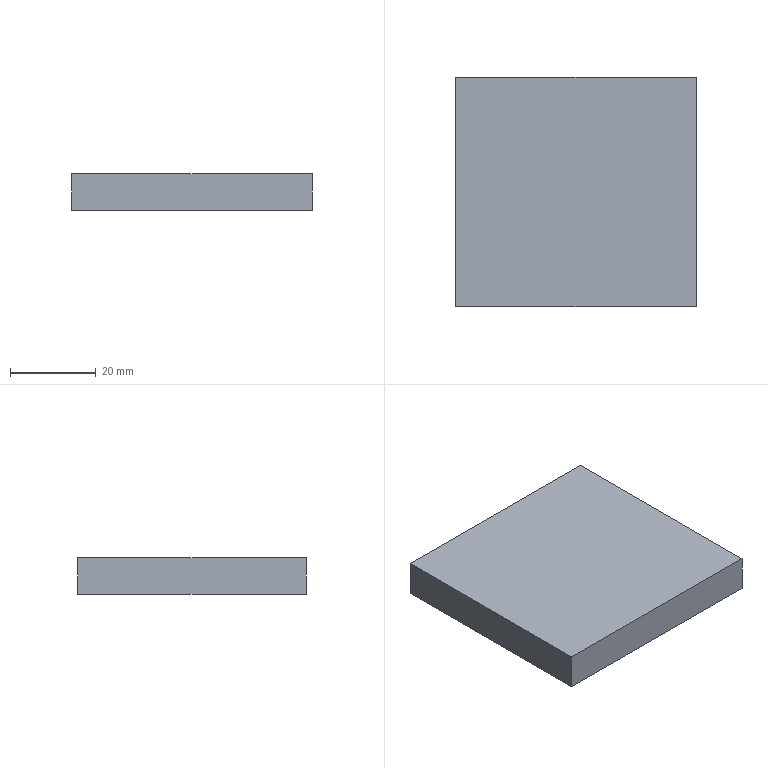NC program | NX | posted with a generic post | part box 56 x 53.3 x 8.5 mm
Lines 2013 to 2943 of 2943:
(ZLEVEL_PROFILE_COPY_COPY_COPY , TOOL : D2)
N4018 T18 M6
N4020 G54
N4022 G17 G0 G90 X19.843 Y-6.394 S9500 M3
N4024 G43 Z30. H18
N4026 Z-0.146
N4028 G94 G1 X20.091 Y-6.597 F1000.
N4030 G3 X20.288 Y-6.629 R0.2
N4032 G2 X21.018 Y-6.5 R2. F1100.
N4034 G3 X21.241 Y-5.728 R22.
N4036 X21.19 Y-5.534 R0.2
N4038 G1 X20.943 Y-5.287
N4040 G0 X19.843 Y-6.394 Z-0.292
N4042 G1 X20.091 Y-6.597 F1000.
N4044 G3 X20.288 Y-6.629 R0.2
N4046 G2 X21.018 Y-6.5 R2. F1100.
N4048 G3 X21.241 Y-5.728 R22.
N4050 X21.19 Y-5.534 R0.2
N4052 G1 X20.943 Y-5.287
N4054 G0 X19.843 Y-6.394 Z-0.438
N4056 G1 X20.091 Y-6.597 F1000.
N4058 G3 X20.288 Y-6.629 R0.2
N4060 G2 X21.018 Y-6.5 R2. F1100.
N4062 G3 X21.241 Y-5.728 R22.
N4064 X21.19 Y-5.534 R0.2
N4066 G1 X20.943 Y-5.287
N4068 G0 X19.843 Y-6.394 Z-0.583
N4070 G1 X20.091 Y-6.597 F1000.
N4072 G3 X20.288 Y-6.629 R0.2
N4074 G2 X21.018 Y-6.5 R2. F1100.
N4076 G3 X21.241 Y-5.728 R22.
N4078 X21.19 Y-5.534 R0.2
N4080 G1 X20.943 Y-5.287
N4082 G0 X19.843 Y-6.394 Z-0.729
N4084 G1 X20.091 Y-6.597 F1000.
N4086 G3 X20.288 Y-6.629 R0.2
N4088 G2 X21.018 Y-6.5 R2. F1100.
N4090 G3 X21.241 Y-5.728 R22.
N4092 X21.19 Y-5.534 R0.2
N4094 G1 X20.943 Y-5.287
N4096 G0 X19.843 Y-6.394 Z-0.875
N4098 G1 X20.091 Y-6.597 F1000.
N4100 G3 X20.288 Y-6.629 R0.2
N4102 G2 X21.018 Y-6.5 R2. F1100.
N4104 G3 X21.241 Y-5.728 R22.
N4106 X21.19 Y-5.534 R0.2
N4108 G1 X20.943 Y-5.287
N4110 G0 X19.843 Y-6.394 Z-1.021
N4112 G1 X20.091 Y-6.597 F1000.
N4114 G3 X20.288 Y-6.629 R0.2
N4116 G2 X21.018 Y-6.5 R2. F1100.
N4118 G3 X21.241 Y-5.728 R22.
N4120 X21.19 Y-5.534 R0.2
N4122 G1 X20.943 Y-5.287
N4124 G0 X19.843 Y-6.394 Z-1.167
N4126 G1 X20.091 Y-6.597 F1000.
N4128 G3 X20.288 Y-6.629 R0.2
N4130 G2 X21.018 Y-6.5 R2. F1100.
N4132 G3 X21.241 Y-5.728 R22.
N4134 X21.19 Y-5.534 R0.2
N4136 G1 X20.943 Y-5.287
N4138 G0 X19.843 Y-6.394 Z-1.313
N4140 G1 X20.091 Y-6.597 F1000.
N4142 G3 X20.288 Y-6.629 R0.2
N4144 G2 X21.018 Y-6.5 R2. F1100.
N4146 G3 X21.241 Y-5.728 R22.
N4148 X21.19 Y-5.534 R0.2
N4150 G1 X20.943 Y-5.287
N4152 G0 X19.843 Y-6.394 Z-1.458
N4154 G1 X20.091 Y-6.597 F1000.
N4156 G3 X20.288 Y-6.629 R0.2
N4158 G2 X21.018 Y-6.5 R2. F1100.
N4160 G3 X21.241 Y-5.728 R22.
N4162 X21.19 Y-5.534 R0.2
N4164 G1 X20.943 Y-5.287
N4166 G0 X19.843 Y-6.394 Z-1.604
N4168 G1 X20.091 Y-6.597 F1000.
N4170 G3 X20.288 Y-6.629 R0.2
N4172 G2 X21.018 Y-6.5 R2. F1100.
N4174 G3 X21.241 Y-5.728 R22.
N4176 X21.19 Y-5.534 R0.2
N4178 G1 X20.943 Y-5.287
N4180 G0 X19.843 Y-6.394 Z-1.75
N4182 G1 X20.091 Y-6.597 F1000.
N4184 G3 X20.288 Y-6.629 R0.2
N4186 G2 X21.018 Y-6.5 R2. F1100.
N4188 G3 X21.241 Y-5.728 R22.
N4190 X21.19 Y-5.534 R0.2
N4192 G1 X20.943 Y-5.287
N4194 G0 X19.843 Y-6.394 Z-1.896
N4196 G1 X20.091 Y-6.597 F1000.
N4198 G3 X20.288 Y-6.629 R0.2
N4200 G2 X21.018 Y-6.5 R2. F1100.
N4202 G3 X21.241 Y-5.728 R22.
N4204 X21.19 Y-5.534 R0.2
N4206 G1 X20.943 Y-5.287
N4208 G0 X19.843 Y-6.394 Z-2.042
N4210 G1 X20.091 Y-6.597 F1000.
N4212 G3 X20.288 Y-6.629 R0.2
N4214 G2 X21.018 Y-6.5 R2. F1100.
N4216 G3 X21.241 Y-5.728 R22.
N4218 X21.19 Y-5.534 R0.2
N4220 G1 X20.943 Y-5.287
N4222 G0 X19.843 Y-6.394 Z-2.188
N4224 G1 X20.091 Y-6.597 F1000.
N4226 G3 X20.288 Y-6.629 R0.2
N4228 G2 X21.018 Y-6.5 R2. F1100.
N4230 G3 X21.241 Y-5.728 R22.
N4232 X21.19 Y-5.534 R0.2
N4234 G1 X20.943 Y-5.287
N4236 G0 X19.843 Y-6.394 Z-2.333
N4238 G1 X20.091 Y-6.597 F1000.
N4240 G3 X20.288 Y-6.629 R0.2
N4242 G2 X21.018 Y-6.5 R2. F1100.
N4244 G3 X21.241 Y-5.728 R22.
N4246 X21.19 Y-5.534 R0.2
N4248 G1 X20.943 Y-5.287
N4250 G0 X19.843 Y-6.394 Z-2.479
N4252 G1 X20.091 Y-6.597 F1000.
N4254 G3 X20.288 Y-6.629 R0.2
N4256 G2 X21.018 Y-6.5 R2. F1100.
N4258 G3 X21.241 Y-5.728 R22.
N4260 X21.19 Y-5.534 R0.2
N4262 G1 X20.943 Y-5.287
N4264 G0 X19.843 Y-6.394 Z-2.625
N4266 G1 X20.091 Y-6.597 F1000.
N4268 G3 X20.288 Y-6.629 R0.2
N4270 G2 X21.018 Y-6.5 R2. F1100.
N4272 G3 X21.241 Y-5.728 R22.
N4274 X21.19 Y-5.534 R0.2
N4276 G1 X20.943 Y-5.287
N4278 G0 X19.843 Y-6.394 Z-2.771
N4280 G1 X20.091 Y-6.597 F1000.
N4282 G3 X20.288 Y-6.629 R0.2
N4284 G2 X21.018 Y-6.5 R2. F1100.
N4286 G3 X21.241 Y-5.728 R22.
N4288 X21.19 Y-5.534 R0.2
N4290 G1 X20.943 Y-5.287
N4292 G0 X19.843 Y-6.394 Z-2.917
N4294 G1 X20.091 Y-6.597 F1000.
N4296 G3 X20.288 Y-6.629 R0.2
N4298 G2 X21.018 Y-6.5 R2. F1100.
N4300 G3 X21.241 Y-5.728 R22.
N4302 X21.19 Y-5.534 R0.2
N4304 G1 X20.943 Y-5.287
N4306 G0 X19.843 Y-6.394 Z-3.063
N4308 G1 X20.091 Y-6.597 F1000.
N4310 G3 X20.288 Y-6.629 R0.2
N4312 G2 X21.018 Y-6.5 R2. F1100.
N4314 G3 X21.241 Y-5.728 R22.
N4316 X21.19 Y-5.534 R0.2
N4318 G1 X20.943 Y-5.287
N4320 G0 X19.843 Y-6.394 Z-3.208
N4322 G1 X20.091 Y-6.597 F1000.
N4324 G3 X20.288 Y-6.629 R0.2
N4326 G2 X21.018 Y-6.5 R2. F1100.
N4328 G3 X21.241 Y-5.728 R22.
N4330 X21.19 Y-5.534 R0.2
N4332 G1 X20.943 Y-5.287
N4334 G0 X19.843 Y-6.394 Z-3.354
N4336 G1 X20.091 Y-6.597 F1000.
N4338 G3 X20.288 Y-6.629 R0.2
N4340 G2 X21.018 Y-6.5 R2. F1100.
N4342 G3 X21.241 Y-5.728 R22.
N4344 X21.19 Y-5.534 R0.2
N4346 G1 X20.943 Y-5.287
N4348 G0 X19.843 Y-6.394 Z-3.5
N4350 G1 X20.091 Y-6.597 F1000.
N4352 G3 X20.288 Y-6.629 R0.2
N4354 G2 X21.018 Y-6.5 R2. F1100.
N4356 G3 X21.241 Y-5.728 R22.
N4358 X21.19 Y-5.534 R0.2
N4360 G1 X20.943 Y-5.287
N4362 G0 Z30.
N4364 Y5.287
N4366 Z-0.146
N4368 G1 X21.19 Y5.534 F1000.
N4370 G3 X21.241 Y5.728 R0.2
N4372 X21.018 Y6.5 R22. F1100.
N4374 G1 X20.995
N4376 G2 X20.288 Y6.629 R2.
N4378 G3 X20.091 Y6.597 R0.2
N4380 G1 X19.843 Y6.394
N4382 G0 X20.943 Y5.287 Z-0.292
N4384 G1 X21.19 Y5.534 F1000.
N4386 G3 X21.241 Y5.728 R0.2
N4388 X21.018 Y6.5 R22. F1100.
N4390 G1 X20.995
N4392 G2 X20.288 Y6.629 R2.
N4394 G3 X20.091 Y6.597 R0.2
N4396 G1 X19.843 Y6.394
N4398 G0 X20.943 Y5.287 Z-0.438
N4400 G1 X21.19 Y5.534 F1000.
N4402 G3 X21.241 Y5.728 R0.2
N4404 X21.018 Y6.5 R22. F1100.
N4406 G1 X20.995
N4408 G2 X20.288 Y6.629 R2.
N4410 G3 X20.091 Y6.597 R0.2
N4412 G1 X19.843 Y6.394
N4414 G0 X20.943 Y5.287 Z-0.583
N4416 G1 X21.19 Y5.534 F1000.
N4418 G3 X21.241 Y5.728 R0.2
N4420 X21.018 Y6.5 R22. F1100.
N4422 G1 X20.995
N4424 G2 X20.288 Y6.629 R2.
N4426 G3 X20.091 Y6.597 R0.2
N4428 G1 X19.843 Y6.394
N4430 G0 X20.943 Y5.287 Z-0.729
N4432 G1 X21.19 Y5.534 F1000.
N4434 G3 X21.241 Y5.728 R0.2
N4436 X21.018 Y6.5 R22. F1100.
N4438 G1 X20.995
N4440 G2 X20.288 Y6.629 R2.
N4442 G3 X20.091 Y6.597 R0.2
N4444 G1 X19.843 Y6.394
N4446 G0 X20.943 Y5.287 Z-0.875
N4448 G1 X21.19 Y5.534 F1000.
N4450 G3 X21.241 Y5.728 R0.2
N4452 X21.018 Y6.5 R22. F1100.
N4454 G1 X20.995
N4456 G2 X20.288 Y6.629 R2.
N4458 G3 X20.091 Y6.597 R0.2
N4460 G1 X19.843 Y6.394
N4462 G0 X20.943 Y5.287 Z-1.021
N4464 G1 X21.19 Y5.534 F1000.
N4466 G3 X21.241 Y5.728 R0.2
N4468 X21.018 Y6.5 R22. F1100.
N4470 G1 X20.995
N4472 G2 X20.288 Y6.629 R2.
N4474 G3 X20.091 Y6.597 R0.2
N4476 G1 X19.843 Y6.394
N4478 G0 X20.943 Y5.287 Z-1.167
N4480 G1 X21.19 Y5.534 F1000.
N4482 G3 X21.241 Y5.728 R0.2
N4484 X21.018 Y6.5 R22. F1100.
N4486 G1 X20.995
N4488 G2 X20.288 Y6.629 R2.
N4490 G3 X20.091 Y6.597 R0.2
N4492 G1 X19.843 Y6.394
N4494 G0 X20.943 Y5.287 Z-1.313
N4496 G1 X21.19 Y5.534 F1000.
N4498 G3 X21.241 Y5.728 R0.2
N4500 X21.018 Y6.5 R22. F1100.
N4502 G1 X20.995
N4504 G2 X20.288 Y6.629 R2.
N4506 G3 X20.091 Y6.597 R0.2
N4508 G1 X19.843 Y6.394
N4510 G0 X20.943 Y5.287 Z-1.458
N4512 G1 X21.19 Y5.534 F1000.
N4514 G3 X21.241 Y5.728 R0.2
N4516 X21.018 Y6.5 R22. F1100.
N4518 G1 X20.995
N4520 G2 X20.288 Y6.629 R2.
N4522 G3 X20.091 Y6.597 R0.2
N4524 G1 X19.843 Y6.394
N4526 G0 X20.943 Y5.287 Z-1.604
N4528 G1 X21.19 Y5.534 F1000.
N4530 G3 X21.241 Y5.728 R0.2
N4532 X21.018 Y6.5 R22. F1100.
N4534 G1 X20.995
N4536 G2 X20.288 Y6.629 R2.
N4538 G3 X20.091 Y6.597 R0.2
N4540 G1 X19.843 Y6.394
N4542 G0 X20.943 Y5.287 Z-1.75
N4544 G1 X21.19 Y5.534 F1000.
N4546 G3 X21.241 Y5.728 R0.2
N4548 X21.018 Y6.5 R22. F1100.
N4550 G1 X20.995
N4552 G2 X20.288 Y6.629 R2.
N4554 G3 X20.091 Y6.597 R0.2
N4556 G1 X19.843 Y6.394
N4558 G0 X20.943 Y5.287 Z-1.896
N4560 G1 X21.19 Y5.534 F1000.
N4562 G3 X21.241 Y5.728 R0.2
N4564 X21.018 Y6.5 R22. F1100.
N4566 G1 X20.995
N4568 G2 X20.288 Y6.629 R2.
N4570 G3 X20.091 Y6.597 R0.2
N4572 G1 X19.843 Y6.394
N4574 G0 X20.943 Y5.287 Z-2.042
N4576 G1 X21.19 Y5.534 F1000.
N4578 G3 X21.241 Y5.728 R0.2
N4580 X21.018 Y6.5 R22. F1100.
N4582 G1 X20.995
N4584 G2 X20.288 Y6.629 R2.
N4586 G3 X20.091 Y6.597 R0.2
N4588 G1 X19.843 Y6.394
N4590 G0 X20.943 Y5.287 Z-2.188
N4592 G1 X21.19 Y5.534 F1000.
N4594 G3 X21.241 Y5.728 R0.2
N4596 X21.018 Y6.5 R22. F1100.
N4598 G1 X20.995
N4600 G2 X20.288 Y6.629 R2.
N4602 G3 X20.091 Y6.597 R0.2
N4604 G1 X19.843 Y6.394
N4606 G0 X20.943 Y5.287 Z-2.333
N4608 G1 X21.19 Y5.534 F1000.
N4610 G3 X21.241 Y5.728 R0.2
N4612 X21.018 Y6.5 R22. F1100.
N4614 G1 X20.995
N4616 G2 X20.288 Y6.629 R2.
N4618 G3 X20.091 Y6.597 R0.2
N4620 G1 X19.843 Y6.394
N4622 G0 X20.943 Y5.287 Z-2.479
N4624 G1 X21.19 Y5.534 F1000.
N4626 G3 X21.241 Y5.728 R0.2
N4628 X21.018 Y6.499 R22. F1100.
N4630 G1 X20.995 Y6.5
N4632 G2 X20.288 Y6.629 R2.
N4634 G3 X20.091 Y6.597 R0.2
N4636 G1 X19.843 Y6.394
N4638 G0 X20.943 Y5.287 Z-2.625
N4640 G1 X21.19 Y5.534 F1000.
N4642 G3 X21.241 Y5.728 R0.2
N4644 X21.018 Y6.499 R22. F1100.
N4646 G1 X20.995 Y6.5
N4648 G2 X20.288 Y6.629 R2.
N4650 G3 X20.091 Y6.597 R0.2
N4652 G1 X19.843 Y6.394
N4654 G0 X20.943 Y5.287 Z-2.771
N4656 G1 X21.19 Y5.534 F1000.
N4658 G3 X21.241 Y5.728 R0.2
N4660 X21.018 Y6.499 R22. F1100.
N4662 G1 X20.995 Y6.5
N4664 G2 X20.288 Y6.629 R2.
N4666 G3 X20.091 Y6.597 R0.2
N4668 G1 X19.843 Y6.394
N4670 G0 X20.943 Y5.287 Z-2.917
N4672 G1 X21.19 Y5.534 F1000.
N4674 G3 X21.241 Y5.728 R0.2
N4676 X21.018 Y6.499 R22. F1100.
N4678 G1 X20.995 Y6.5
N4680 G2 X20.288 Y6.629 R2.
N4682 G3 X20.091 Y6.597 R0.2
N4684 G1 X19.843 Y6.394
N4686 G0 X20.943 Y5.287 Z-3.063
N4688 G1 X21.19 Y5.534 F1000.
N4690 G3 X21.241 Y5.728 R0.2
N4692 X21.018 Y6.499 R22. F1100.
N4694 G1 X20.995 Y6.5
N4696 G2 X20.288 Y6.629 R2.
N4698 G3 X20.091 Y6.597 R0.2
N4700 G1 X19.843 Y6.394
N4702 G0 X20.943 Y5.287 Z-3.208
N4704 G1 X21.19 Y5.534 F1000.
N4706 G3 X21.241 Y5.728 R0.2
N4708 X21.018 Y6.499 R22. F1100.
N4710 G1 X20.995 Y6.5
N4712 G2 X20.288 Y6.629 R2.
N4714 G3 X20.091 Y6.597 R0.2
N4716 G1 X19.843 Y6.394
N4718 G0 X20.943 Y5.287 Z-3.354
N4720 G1 X21.19 Y5.534 F1000.
N4722 G3 X21.241 Y5.728 R0.2
N4724 X21.018 Y6.499 R22. F1100.
N4726 G1 X20.995 Y6.5
N4728 G2 X20.288 Y6.629 R2.
N4730 G3 X20.091 Y6.597 R0.2
N4732 G1 X19.843 Y6.394
N4734 G0 X20.943 Y5.287 Z-3.5
N4736 G1 X21.19 Y5.534 F1000.
N4738 G3 X21.241 Y5.728 R0.2
N4740 X21.018 Y6.499 R22. F1100.
N4742 G1 X20.995 Y6.5
N4744 G2 X20.288 Y6.629 R2.
N4746 G3 X20.091 Y6.597 R0.2
N4748 G1 X19.843 Y6.394
N4750 G0 Z30.
N4752 X-19.843
N4754 Z-0.146
N4756 G1 X-20.091 Y6.597 F1000.
N4758 G3 X-20.288 Y6.629 R0.2
N4760 G2 X-21.018 Y6.5 R2. F1100.
N4762 G3 X-21.241 Y5.728 R22.
N4764 X-21.19 Y5.534 R0.2
N4766 G1 X-20.943 Y5.287
N4768 G0 X-19.843 Y6.394 Z-0.292
N4770 G1 X-20.091 Y6.597 F1000.
N4772 G3 X-20.288 Y6.629 R0.2
N4774 G2 X-21.018 Y6.5 R2. F1100.
N4776 G3 X-21.241 Y5.728 R22.
N4778 X-21.19 Y5.534 R0.2
N4780 G1 X-20.943 Y5.287
N4782 G0 X-19.843 Y6.394 Z-0.438
N4784 G1 X-20.091 Y6.597 F1000.
N4786 G3 X-20.288 Y6.629 R0.2
N4788 G2 X-21.018 Y6.5 R2. F1100.
N4790 G3 X-21.241 Y5.728 R22.
N4792 X-21.19 Y5.534 R0.2
N4794 G1 X-20.943 Y5.287
N4796 G0 X-19.843 Y6.394 Z-0.583
N4798 G1 X-20.091 Y6.597 F1000.
N4800 G3 X-20.288 Y6.629 R0.2
N4802 G2 X-21.018 Y6.5 R2. F1100.
N4804 G3 X-21.241 Y5.728 R22.
N4806 X-21.19 Y5.534 R0.2
N4808 G1 X-20.943 Y5.287
N4810 G0 X-19.843 Y6.394 Z-0.729
N4812 G1 X-20.091 Y6.597 F1000.
N4814 G3 X-20.288 Y6.629 R0.2
N4816 G2 X-21.018 Y6.5 R2. F1100.
N4818 G3 X-21.241 Y5.728 R22.
N4820 X-21.19 Y5.534 R0.2
N4822 G1 X-20.943 Y5.287
N4824 G0 X-19.843 Y6.394 Z-0.875
N4826 G1 X-20.091 Y6.597 F1000.
N4828 G3 X-20.288 Y6.629 R0.2
N4830 G2 X-21.018 Y6.5 R2. F1100.
N4832 G3 X-21.241 Y5.728 R22.
N4834 X-21.19 Y5.534 R0.2
N4836 G1 X-20.943 Y5.287
N4838 G0 X-19.843 Y6.394 Z-1.021
N4840 G1 X-20.091 Y6.597 F1000.
N4842 G3 X-20.288 Y6.629 R0.2
N4844 G2 X-21.018 Y6.5 R2. F1100.
N4846 G3 X-21.241 Y5.728 R22.
N4848 X-21.19 Y5.534 R0.2
N4850 G1 X-20.943 Y5.287
N4852 G0 X-19.843 Y6.394 Z-1.167
N4854 G1 X-20.091 Y6.597 F1000.
N4856 G3 X-20.288 Y6.629 R0.2
N4858 G2 X-21.018 Y6.5 R2. F1100.
N4860 G3 X-21.241 Y5.728 R22.
N4862 X-21.19 Y5.534 R0.2
N4864 G1 X-20.943 Y5.287
N4866 G0 X-19.843 Y6.394 Z-1.313
N4868 G1 X-20.091 Y6.597 F1000.
N4870 G3 X-20.288 Y6.629 R0.2
N4872 G2 X-21.018 Y6.5 R2. F1100.
N4874 G3 X-21.241 Y5.728 R22.
N4876 X-21.19 Y5.534 R0.2
N4878 G1 X-20.943 Y5.287
N4880 G0 X-19.843 Y6.394 Z-1.458
N4882 G1 X-20.091 Y6.597 F1000.
N4884 G3 X-20.288 Y6.629 R0.2
N4886 G2 X-21.018 Y6.5 R2. F1100.
N4888 G3 X-21.241 Y5.728 R22.
N4890 X-21.19 Y5.534 R0.2
N4892 G1 X-20.943 Y5.287
N4894 G0 X-19.843 Y6.394 Z-1.604
N4896 G1 X-20.091 Y6.597 F1000.
N4898 G3 X-20.288 Y6.629 R0.2
N4900 G2 X-21.018 Y6.5 R2. F1100.
N4902 G3 X-21.241 Y5.728 R22.
N4904 X-21.19 Y5.534 R0.2
N4906 G1 X-20.943 Y5.287
N4908 G0 X-19.843 Y6.394 Z-1.75
N4910 G1 X-20.091 Y6.597 F1000.
N4912 G3 X-20.288 Y6.629 R0.2
N4914 G2 X-21.018 Y6.5 R2. F1100.
N4916 G3 X-21.241 Y5.728 R22.
N4918 X-21.19 Y5.534 R0.2
N4920 G1 X-20.943 Y5.287
N4922 G0 X-19.843 Y6.394 Z-1.896
N4924 G1 X-20.091 Y6.597 F1000.
N4926 G3 X-20.288 Y6.629 R0.2
N4928 G2 X-21.018 Y6.5 R2. F1100.
N4930 G3 X-21.241 Y5.728 R22.
N4932 X-21.19 Y5.534 R0.2
N4934 G1 X-20.943 Y5.287
N4936 G0 X-19.843 Y6.394 Z-2.042
N4938 G1 X-20.091 Y6.597 F1000.
N4940 G3 X-20.288 Y6.629 R0.2
N4942 G2 X-21.018 Y6.5 R2.001 F1100.
N4944 G3 X-21.241 Y5.728 R22.
N4946 X-21.19 Y5.534 R0.2
N4948 G1 X-20.943 Y5.287
N4950 G0 X-19.843 Y6.394 Z-2.188
N4952 G1 X-20.091 Y6.597 F1000.
N4954 G3 X-20.288 Y6.629 R0.2
N4956 G2 X-21.018 Y6.5 R2.001 F1100.
N4958 G3 X-21.241 Y5.728 R22.
N4960 X-21.19 Y5.534 R0.2
N4962 G1 X-20.943 Y5.287
N4964 G0 X-19.843 Y6.394 Z-2.333
N4966 G1 X-20.091 Y6.597 F1000.
N4968 G3 X-20.288 Y6.629 R0.2
N4970 G2 X-21.018 Y6.5 R2.001 F1100.
N4972 G3 X-21.241 Y5.728 R22.
N4974 X-21.19 Y5.534 R0.2
N4976 G1 X-20.943 Y5.287
N4978 G0 X-19.843 Y6.394 Z-2.479
N4980 G1 X-20.091 Y6.597 F1000.
N4982 G3 X-20.288 Y6.629 R0.2
N4984 G2 X-21.018 Y6.499 R2.001 F1100.
N4986 G3 X-21.241 Y5.728 R22.
N4988 X-21.19 Y5.534 R0.2
N4990 G1 X-20.943 Y5.287
N4992 G0 X-19.843 Y6.394 Z-2.625
N4994 G1 X-20.091 Y6.597 F1000.
N4996 G3 X-20.288 Y6.629 R0.2
N4998 G2 X-21.018 Y6.499 R2.001 F1100.
N5000 G3 X-21.241 Y5.728 R22.
N5002 X-21.19 Y5.534 R0.2
N5004 G1 X-20.943 Y5.287
N5006 G0 X-19.843 Y6.394 Z-2.771
N5008 G1 X-20.091 Y6.597 F1000.
N5010 G3 X-20.288 Y6.629 R0.2
N5012 G2 X-21.018 Y6.499 R2.001 F1100.
N5014 G3 X-21.241 Y5.728 R22.
N5016 X-21.19 Y5.534 R0.2
N5018 G1 X-20.943 Y5.287
N5020 G0 X-19.843 Y6.394 Z-2.917
N5022 G1 X-20.091 Y6.597 F1000.
N5024 G3 X-20.288 Y6.629 R0.2
N5026 G2 X-21.018 Y6.499 R2.001 F1100.
N5028 G3 X-21.241 Y5.728 R22.
N5030 X-21.19 Y5.534 R0.2
N5032 G1 X-20.943 Y5.287
N5034 G0 X-19.843 Y6.394 Z-3.063
N5036 G1 X-20.091 Y6.597 F1000.
N5038 G3 X-20.288 Y6.629 R0.2
N5040 G2 X-21.018 Y6.499 R2.001 F1100.
N5042 G3 X-21.241 Y5.728 R22.
N5044 X-21.19 Y5.534 R0.2
N5046 G1 X-20.943 Y5.287
N5048 G0 X-19.843 Y6.394 Z-3.208
N5050 G1 X-20.091 Y6.597 F1000.
N5052 G3 X-20.288 Y6.629 R0.2
N5054 G2 X-21.018 Y6.499 R2.001 F1100.
N5056 G3 X-21.241 Y5.728 R22.
N5058 X-21.19 Y5.534 R0.2
N5060 G1 X-20.943 Y5.287
N5062 G0 X-19.843 Y6.394 Z-3.354
N5064 G1 X-20.091 Y6.597 F1000.
N5066 G3 X-20.288 Y6.629 R0.2
N5068 G2 X-21.018 Y6.499 R2.001 F1100.
N5070 G3 X-21.241 Y5.728 R22.
N5072 X-21.19 Y5.534 R0.2
N5074 G1 X-20.943 Y5.287
N5076 G0 X-19.843 Y6.394 Z-3.5
N5078 G1 X-20.091 Y6.597 F1000.
N5080 G3 X-20.288 Y6.629 R0.2
N5082 G2 X-21.018 Y6.499 R2.001 F1100.
N5084 G3 X-21.241 Y5.728 R22.
N5086 X-21.19 Y5.534 R0.2
N5088 G1 X-20.943 Y5.287
N5090 G0 Z30.
N5092 Y-5.287
N5094 Z-0.146
N5096 G1 X-21.19 Y-5.534 F1000.
N5098 G3 X-21.241 Y-5.728 R0.2
N5100 X-21.018 Y-6.5 R22. F1100.
N5102 G1 X-20.995
N5104 G2 X-20.288 Y-6.629 R2.
N5106 G3 X-20.091 Y-6.597 R0.2
N5108 G1 X-19.843 Y-6.394
N5110 G0 X-20.943 Y-5.287 Z-0.292
N5112 G1 X-21.19 Y-5.534 F1000.
N5114 G3 X-21.241 Y-5.728 R0.2
N5116 X-21.018 Y-6.5 R22. F1100.
N5118 G1 X-20.995
N5120 G2 X-20.288 Y-6.629 R2.
N5122 G3 X-20.091 Y-6.597 R0.2
N5124 G1 X-19.843 Y-6.394
N5126 G0 X-20.943 Y-5.287 Z-0.438
N5128 G1 X-21.19 Y-5.534 F1000.
N5130 G3 X-21.241 Y-5.728 R0.2
N5132 X-21.018 Y-6.5 R22. F1100.
N5134 G1 X-20.995
N5136 G2 X-20.288 Y-6.629 R2.
N5138 G3 X-20.091 Y-6.597 R0.2
N5140 G1 X-19.843 Y-6.394
N5142 G0 X-20.943 Y-5.287 Z-0.583
N5144 G1 X-21.19 Y-5.534 F1000.
N5146 G3 X-21.241 Y-5.728 R0.2
N5148 X-21.018 Y-6.5 R22. F1100.
N5150 G1 X-20.995
N5152 G2 X-20.288 Y-6.629 R2.
N5154 G3 X-20.091 Y-6.597 R0.2
N5156 G1 X-19.843 Y-6.394
N5158 G0 X-20.943 Y-5.287 Z-0.729
N5160 G1 X-21.19 Y-5.534 F1000.
N5162 G3 X-21.241 Y-5.728 R0.2
N5164 X-21.018 Y-6.5 R22. F1100.
N5166 G1 X-20.995
N5168 G2 X-20.288 Y-6.629 R2.
N5170 G3 X-20.091 Y-6.597 R0.2
N5172 G1 X-19.843 Y-6.394
N5174 G0 X-20.943 Y-5.287 Z-0.875
N5176 G1 X-21.19 Y-5.534 F1000.
N5178 G3 X-21.241 Y-5.728 R0.2
N5180 X-21.018 Y-6.5 R22. F1100.
N5182 G1 X-20.995
N5184 G2 X-20.288 Y-6.629 R2.
N5186 G3 X-20.091 Y-6.597 R0.2
N5188 G1 X-19.843 Y-6.394
N5190 G0 X-20.943 Y-5.287 Z-1.021
N5192 G1 X-21.19 Y-5.534 F1000.
N5194 G3 X-21.241 Y-5.728 R0.2
N5196 X-21.018 Y-6.5 R22. F1100.
N5198 G1 X-20.995
N5200 G2 X-20.288 Y-6.629 R2.
N5202 G3 X-20.091 Y-6.597 R0.2
N5204 G1 X-19.843 Y-6.394
N5206 G0 X-20.943 Y-5.287 Z-1.167
N5208 G1 X-21.19 Y-5.534 F1000.
N5210 G3 X-21.241 Y-5.728 R0.2
N5212 X-21.018 Y-6.5 R22. F1100.
N5214 G1 X-20.995
N5216 G2 X-20.288 Y-6.629 R2.
N5218 G3 X-20.091 Y-6.597 R0.2
N5220 G1 X-19.843 Y-6.394
N5222 G0 X-20.943 Y-5.287 Z-1.313
N5224 G1 X-21.19 Y-5.534 F1000.
N5226 G3 X-21.241 Y-5.728 R0.2
N5228 X-21.018 Y-6.5 R22. F1100.
N5230 G1 X-20.995
N5232 G2 X-20.288 Y-6.629 R2.
N5234 G3 X-20.091 Y-6.597 R0.2
N5236 G1 X-19.843 Y-6.394
N5238 G0 X-20.943 Y-5.287 Z-1.458
N5240 G1 X-21.19 Y-5.534 F1000.
N5242 G3 X-21.241 Y-5.728 R0.2
N5244 X-21.018 Y-6.5 R22. F1100.
N5246 G1 X-20.995
N5248 G2 X-20.288 Y-6.629 R2.
N5250 G3 X-20.091 Y-6.597 R0.2
N5252 G1 X-19.843 Y-6.394
N5254 G0 X-20.943 Y-5.287 Z-1.604
N5256 G1 X-21.19 Y-5.534 F1000.
N5258 G3 X-21.241 Y-5.728 R0.2
N5260 X-21.018 Y-6.5 R22. F1100.
N5262 G1 X-20.995
N5264 G2 X-20.288 Y-6.629 R2.
N5266 G3 X-20.091 Y-6.597 R0.2
N5268 G1 X-19.843 Y-6.394
N5270 G0 X-20.943 Y-5.287 Z-1.75
N5272 G1 X-21.19 Y-5.534 F1000.
N5274 G3 X-21.241 Y-5.728 R0.2
N5276 X-21.018 Y-6.5 R22. F1100.
N5278 G1 X-20.995
N5280 G2 X-20.288 Y-6.629 R2.
N5282 G3 X-20.091 Y-6.597 R0.2
N5284 G1 X-19.843 Y-6.394
N5286 G0 X-20.943 Y-5.287 Z-1.896
N5288 G1 X-21.19 Y-5.534 F1000.
N5290 G3 X-21.241 Y-5.728 R0.2
N5292 X-21.018 Y-6.5 R22. F1100.
N5294 G1 X-20.995
N5296 G2 X-20.288 Y-6.629 R2.
N5298 G3 X-20.091 Y-6.597 R0.2
N5300 G1 X-19.843 Y-6.394
N5302 G0 X-20.943 Y-5.287 Z-2.042
N5304 G1 X-21.19 Y-5.534 F1000.
N5306 G3 X-21.241 Y-5.728 R0.2
N5308 X-21.018 Y-6.5 R22. F1100.
N5310 G1 X-20.995
N5312 G2 X-20.288 Y-6.629 R2.
N5314 G3 X-20.091 Y-6.597 R0.2
N5316 G1 X-19.843 Y-6.394
N5318 G0 X-20.943 Y-5.287 Z-2.188
N5320 G1 X-21.19 Y-5.534 F1000.
N5322 G3 X-21.241 Y-5.728 R0.2
N5324 X-21.018 Y-6.5 R22. F1100.
N5326 G1 X-20.995
N5328 G2 X-20.288 Y-6.629 R2.
N5330 G3 X-20.091 Y-6.597 R0.2
N5332 G1 X-19.843 Y-6.394
N5334 G0 X-20.943 Y-5.287 Z-2.333
N5336 G1 X-21.19 Y-5.534 F1000.
N5338 G3 X-21.241 Y-5.728 R0.2
N5340 X-21.018 Y-6.5 R22. F1100.
N5342 G1 X-20.995
N5344 G2 X-20.288 Y-6.629 R2.
N5346 G3 X-20.091 Y-6.597 R0.2
N5348 G1 X-19.843 Y-6.394
N5350 G0 X-20.943 Y-5.287 Z-2.479
N5352 G1 X-21.19 Y-5.534 F1000.
N5354 G3 X-21.241 Y-5.728 R0.2
N5356 X-21.018 Y-6.5 R22. F1100.
N5358 G1 X-20.995
N5360 G2 X-20.288 Y-6.629 R2.
N5362 G3 X-20.091 Y-6.597 R0.2
N5364 G1 X-19.843 Y-6.394
N5366 G0 X-20.943 Y-5.287 Z-2.625
N5368 G1 X-21.19 Y-5.534 F1000.
N5370 G3 X-21.241 Y-5.728 R0.2
N5372 X-21.018 Y-6.5 R22. F1100.
N5374 G1 X-20.995
N5376 G2 X-20.288 Y-6.629 R2.
N5378 G3 X-20.091 Y-6.597 R0.2
N5380 G1 X-19.843 Y-6.394
N5382 G0 X-20.943 Y-5.287 Z-2.771
N5384 G1 X-21.19 Y-5.534 F1000.
N5386 G3 X-21.241 Y-5.728 R0.2
N5388 X-21.018 Y-6.5 R22. F1100.
N5390 G1 X-20.995
N5392 G2 X-20.288 Y-6.629 R2.
N5394 G3 X-20.091 Y-6.597 R0.2
N5396 G1 X-19.843 Y-6.394
N5398 G0 X-20.943 Y-5.287 Z-2.917
N5400 G1 X-21.19 Y-5.534 F1000.
N5402 G3 X-21.241 Y-5.728 R0.2
N5404 X-21.018 Y-6.5 R22. F1100.
N5406 G1 X-20.995
N5408 G2 X-20.288 Y-6.629 R2.
N5410 G3 X-20.091 Y-6.597 R0.2
N5412 G1 X-19.843 Y-6.394
N5414 G0 X-20.943 Y-5.287 Z-3.063
N5416 G1 X-21.19 Y-5.534 F1000.
N5418 G3 X-21.241 Y-5.728 R0.2
N5420 X-21.018 Y-6.5 R22. F1100.
N5422 G1 X-20.995
N5424 G2 X-20.288 Y-6.629 R2.
N5426 G3 X-20.091 Y-6.597 R0.2
N5428 G1 X-19.843 Y-6.394
N5430 G0 X-20.943 Y-5.287 Z-3.208
N5432 G1 X-21.19 Y-5.534 F1000.
N5434 G3 X-21.241 Y-5.728 R0.2
N5436 X-21.018 Y-6.5 R22. F1100.
N5438 G1 X-20.995
N5440 G2 X-20.288 Y-6.629 R2.
N5442 G3 X-20.091 Y-6.597 R0.2
N5444 G1 X-19.843 Y-6.394
N5446 G0 X-20.943 Y-5.287 Z-3.354
N5448 G1 X-21.19 Y-5.534 F1000.
N5450 G3 X-21.241 Y-5.728 R0.2
N5452 X-21.018 Y-6.5 R22. F1100.
N5454 G1 X-20.995
N5456 G2 X-20.288 Y-6.629 R2.
N5458 G3 X-20.091 Y-6.597 R0.2
N5460 G1 X-19.843 Y-6.394
N5462 G0 X-20.943 Y-5.287 Z-3.5
N5464 G1 X-21.19 Y-5.534 F1000.
N5466 G3 X-21.241 Y-5.728 R0.2
N5468 X-21.018 Y-6.5 R22. F1100.
N5470 G1 X-20.995
N5472 G2 X-20.288 Y-6.629 R2.
N5474 G3 X-20.091 Y-6.597 R0.2
N5476 G1 X-19.843 Y-6.394
N5478 G0 Z30.
N5480 M5
(FLOOR_WALL_COPY_1 , TOOL : D4)
N5482 T11 M6
N5484 G54
N5486 G17 G0 G90 X2.008 Y-0.769 S9500 M3
N5488 G43 Z30. H11
N5490 Z-0.4
N5492 G94 G1 X2.455 Y-0.373 Z-0.56 F1100.
N5494 X2.926 Y0. Z-0.721
N5496 X2.455 Y0.373 Z-0.882
N5498 X1.904 Y0.861 Z-1.079
N5500 X0.861 Y1.904 Z-1.474
N5502 X0.373 Y2.455 Z-1.672
N5504 X0. Y2.926 Z-1.833
N5506 X-0.373 Y2.455 Z-1.994
N5508 X-0.861 Y1.904 Z-2.191
N5510 X-1.904 Y0.861 Z-2.586
N5512 X-2.455 Y0.373 Z-2.783
N5514 X-2.926 Y0. Z-2.944
N5516 X-2.455 Y-0.373 Z-3.105
N5518 X-1.904 Y-0.861 Z-3.302
N5520 X-1.379 Y-1.379 Z-3.5
N5522 X-0.106 Y-0.106
N5524 X0. Y-0.213
N5526 G2 X0.213 Y0. R19.85
N5528 X0. Y0.213 R19.85
N5530 X-0.213 Y0. R19.85
N5532 G1 X-0.106 Y-0.106
N5534 X-1.379 Y-1.379
N5536 G2 X0. Y-2.926 R18.05
N5538 X2.926 Y0. R18.05
N5540 X0. Y2.926 R18.05
N5542 X-2.926 Y0. R18.05
N5544 X-1.379 Y-1.379 R18.05
N5546 G1 X-2.793 Y-2.793
N5548 G2 X0. Y-6.553 R16.05
N5550 X6.553 Y0. R16.05
N5552 X0. Y6.553 R16.05
N5554 X-6.553 Y0. R16.05
N5556 X-2.793 Y-2.793 R16.05
N5558 G1 X-4.207 Y-4.207
N5560 G2 X-0.842 Y-9.613 R14.05
N5562 G3 X0.842 Y-9.613 R9.65
N5564 G2 X10.74 Y-0.51 R14.05
N5566 X10.998 Y-0.189 R13.
N5568 G3 X10.998 Y0.189 R11.
N5570 G2 X10.74 Y0.51 R13.
N5572 X0.842 Y9.613 R14.05
N5574 G3 X-0.842 Y9.613 R9.65
N5576 G2 X-10.74 Y0.51 R14.05
N5578 X-10.998 Y0.189 R13.
N5580 G3 X-10.998 Y-0.189 R11.
N5582 G2 X-10.74 Y-0.51 R13.
N5584 X-4.207 Y-4.207 R14.05
N5586 G1 X-5.621 Y-5.621
N5588 G2 X-2.409 Y-11.398 R12.05
N5590 G3 X2.409 Y-11.398 R11.65
N5592 G2 X11.908 Y-2.301 R12.05
N5594 X12.963 Y-0.984 R11.
N5596 G3 X12.963 Y0.984 R13.
N5598 G2 X11.908 Y2.301 R11.
N5600 X2.409 Y11.398 R12.05
N5602 G3 X-2.409 Y11.398 R11.65
N5604 G2 X-11.908 Y2.301 R12.05
N5606 X-12.963 Y0.984 R11.
N5608 G3 X-12.963 Y-0.984 R13.
N5610 G2 X-11.908 Y-2.301 R11.
N5612 X-5.621 Y-5.621 R12.05
N5614 G1 X-7.036 Y-7.036
N5616 G2 X-4.157 Y-13.002 R10.05
N5618 G3 X4.157 Y-13.002 R13.65
N5620 G2 X13.119 Y-4.144 R10.05
N5622 X14.88 Y-1.896 R9.
N5624 G3 X14.88 Y1.896 R15.
N5626 G2 X13.119 Y4.144 R9.
N5628 X4.157 Y13.002 R10.05
N5630 G3 X-4.157 Y13.002 R13.65
N5632 G2 X-13.119 Y4.144 R10.05
N5634 X-14.88 Y1.896 R9.
N5636 G3 X-14.88 Y-1.896 R15.
N5638 G2 X-13.119 Y-4.144 R9.
N5640 X-7.036 Y-7.036 R10.05
N5642 G1 X-8.45 Y-8.45
N5644 G2 X-6.097 Y-14.414 R8.05
N5646 G3 X6.097 Y-14.414 R15.65
N5648 G2 X14.414 Y-6.097 R8.05
N5650 G3 X14.506 Y-5.873 R15.65
N5652 G2 X16.744 Y-2.938 R7.
N5654 G3 X16.744 Y2.938 R17.
N5656 G2 X14.506 Y5.873 R7.
N5658 G3 X14.414 Y6.097 R15.65
N5660 G2 X6.097 Y14.414 R8.05
N5662 G3 X-6.097 Y14.414 R15.65
N5664 G2 X-14.414 Y6.097 R8.05
N5666 G3 X-14.506 Y5.873 R15.65
N5668 G2 X-16.744 Y2.938 R7.
N5670 G3 X-16.744 Y-2.938 R17.
N5672 G2 X-14.506 Y-5.873 R7.
N5674 G3 X-14.414 Y-6.097 R15.65
N5676 G2 X-8.45 Y-8.45 R8.05
N5678 G1 X-9.864 Y-9.864
N5680 G2 X-8.269 Y-15.593 R6.05
N5682 G3 X8.269 Y-15.593 R17.65
N5684 G2 X15.593 Y-8.269 R6.05
N5686 G3 X16.36 Y-6.624 R17.65
N5688 G2 X18.543 Y-4.142 R5.
N5690 G3 X18.543 Y4.142 R19.
N5692 G2 X16.36 Y6.624 R5.
N5694 G3 X15.593 Y8.269 R17.65
N5696 G2 X8.269 Y15.593 R6.05
N5698 G3 X-8.269 Y15.593 R17.65
N5700 G2 X-15.593 Y8.269 R6.05
N5702 G3 X-16.36 Y6.624 R17.65
N5704 G2 X-18.543 Y4.142 R5.
N5706 G3 X-18.543 Y-4.142 R19.
N5708 G2 X-16.36 Y-6.624 R5.
N5710 G3 X-15.593 Y-8.269 R17.65
N5712 G2 X-9.864 Y-9.864 R6.05
N5714 G1 X-11.278 Y-11.278
N5716 G2 X-10.558 Y-16.028 R4.05
N5718 G3 X-10.379 Y-16.685 R0.5
N5720 X10.379 Y-16.685 R19.65
N5722 X10.558 Y-16.028 R0.5
N5724 G2 X16.028 Y-10.558 R4.05
N5726 G3 X16.685 Y-10.379 R0.5
N5728 X18.214 Y-7.374 R19.65
N5730 G2 X20.241 Y-5.596 R3.
N5732 G3 X20.241 Y5.596 R21.
N5734 G2 X18.214 Y7.374 R3.
N5736 G3 X16.685 Y10.379 R19.65
N5738 X16.028 Y10.558 R0.5
N5740 G2 X10.558 Y16.028 R4.05
N5742 G3 X10.379 Y16.685 R0.5
N5744 X-10.379 Y16.685 R19.65
N5746 X-10.558 Y16.028 R0.5
N5748 G2 X-16.028 Y10.558 R4.05
N5750 G3 X-16.685 Y10.379 R0.5
N5752 X-18.214 Y7.374 R19.65
N5754 G2 X-20.241 Y5.596 R3.
N5756 G3 X-20.241 Y-5.596 R21.
N5758 G2 X-18.214 Y-7.374 R3.
N5760 G3 X-16.685 Y-10.379 R19.65
N5762 X-16.028 Y-10.558 R0.5
N5764 G2 X-11.278 Y-11.278 R4.05
N5766 G1 X-9.157 Y-9.157
N5768 Z-0.5
N5770 G0 Z30.
N5772 M5
(刀补11_COPY , TOOL : D2)
N5774 T18 M6
N5776 G54
N5778 G17 G0 G90 X-16.832 Y10.967 S9500 M3
N5780 G43 Z30. H18
N5782 Z-2.5
N5784 G94 G1 Z-3.5 F1000.
N5786 G41 X-16.93 Y10.988 D18
N5788 X-17.358 Y11.002
N5790 G3 X-17.534 Y10.908 R0.2
N5792 X-19.141 Y7.749 R20.65 F1200.
N5794 G2 X-21.018 Y6.5 R2.
N5796 G3 X-21.018 Y-6.5 R22.
N5798 G1 X-20.995
N5800 G2 X-19.141 Y-7.749 R2.
N5802 G3 X-17.534 Y-10.908 R20.65
N5804 X-15.562 Y-11.443 R1.5
N5806 G2 X-11.443 Y-15.562 R3.05
N5808 G3 X-10.908 Y-17.534 R1.5
N5810 X10.908 Y-17.534 R20.65
N5812 X11.443 Y-15.562 R1.5
N5814 G2 X15.562 Y-11.443 R3.05
N5816 G3 X17.534 Y-10.908 R1.5
N5818 X19.141 Y-7.749 R20.65
N5820 G2 X21.009 Y-6.5 R2.
N5822 G1 X21.028 Y-6.468
N5824 G3 X21.018 Y6.5 R22.
N5826 G1 X20.995
N5828 G2 X19.141 Y7.749 R2.
N5830 G3 X17.534 Y10.908 R20.65
N5832 X15.562 Y11.443 R1.5
N5834 G2 X11.443 Y15.562 R3.05
N5836 G3 X10.908 Y17.534 R1.5
N5838 X-10.908 Y17.534 R20.65
N5840 X-11.443 Y15.562 R1.5
N5842 G2 X-15.562 Y11.443 R3.05
N5844 G3 X-17.534 Y10.908 R1.5
N5846 X-17.541 Y10.708 R0.2
N5848 G1 X-17.376 Y10.399
N5850 G40
N5852 X-17.314 Y10.32
N5854 Z-2.5
N5856 G0 Z30.
N5858 M5
N5860 M2